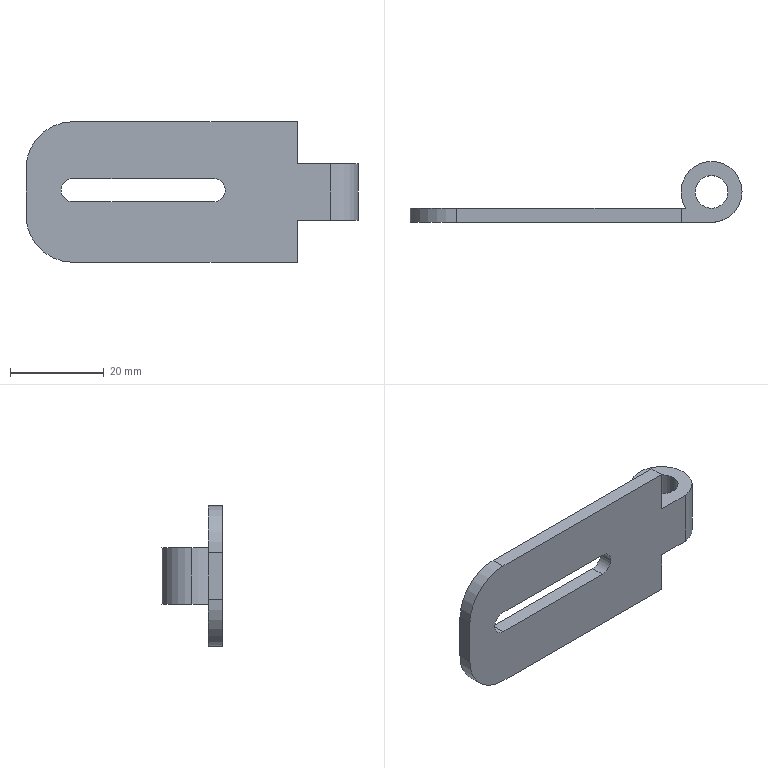Part | SolidWorks | features ICE 2, Extrusion 1, Fillet 1 | 1 solid | 20 faces | box 70.865 x 12.969 x 30 mm | volume 5794 mm3 | plane 11 | cylinder 9 | commonest cylinder face diameters 13 x3 5 x2 7 x2 20 x2
STEP:
#1=CARTESIAN_POINT('',(35.365,4.969,21.));
#2=VERTEX_POINT('',#1);
#3=CARTESIAN_POINT('',(28.365,4.969,21.));
#4=VERTEX_POINT('',#3);
#5=CARTESIAN_POINT('',(31.865,4.969,21.));
#6=DIRECTION('',(0.,0.,-1.));
#7=DIRECTION('',(-1.,0.,0.));
#8=AXIS2_PLACEMENT_3D('',#5,#6,#7);
#9=CIRCLE('',#8,3.5);
#10=EDGE_CURVE('',#2,#4,#9,.T.);
#11=ORIENTED_EDGE('',*,*,#10,.F.);
#12=CARTESIAN_POINT('',(35.365,4.969,9.));
#13=VERTEX_POINT('',#12);
#14=CARTESIAN_POINT('',(35.365,4.969,30.));
#15=DIRECTION('',(0.,0.,-1.));
#16=VECTOR('',#15,1000.);
#17=LINE('',#14,#16);
#18=EDGE_CURVE('',#2,#13,#17,.T.);
#19=ORIENTED_EDGE('',*,*,#18,.T.);
#20=CARTESIAN_POINT('',(28.365,4.969,9.));
#21=VERTEX_POINT('',#20);
#22=CARTESIAN_POINT('',(31.865,4.969,9.));
#23=DIRECTION('',(0.,0.,1.));
#24=DIRECTION('',(1.,0.,0.));
#25=AXIS2_PLACEMENT_3D('',#22,#23,#24);
#26=CIRCLE('',#25,3.5);
#27=EDGE_CURVE('',#21,#13,#26,.T.);
#28=ORIENTED_EDGE('',*,*,#27,.F.);
#29=CARTESIAN_POINT('',(28.365,4.969,30.));
#30=DIRECTION('',(0.,0.,-1.));
#31=VECTOR('',#30,1000.);
#32=LINE('',#29,#31);
#33=EDGE_CURVE('',#4,#21,#32,.T.);
#34=ORIENTED_EDGE('',*,*,#33,.F.);
#35=EDGE_LOOP('',(#11,#19,#28,#34));
#36=FACE_OUTER_BOUND('',#35,.T.);
#37=CARTESIAN_POINT('',(31.865,4.969,30.));
#38=DIRECTION('',(0.,0.,-1.));
#39=DIRECTION('',(-1.,0.,0.));
#40=AXIS2_PLACEMENT_3D('',#37,#38,#39);
#41=CYLINDRICAL_SURFACE('',#40,3.5);
#42=ADVANCED_FACE('',(#36),#41,.F.);
#43=CARTESIAN_POINT('',(25.365,4.969,21.));
#44=VERTEX_POINT('',#43);
#45=CARTESIAN_POINT('',(38.365,4.969,21.));
#46=VERTEX_POINT('',#45);
#47=CARTESIAN_POINT('',(31.865,4.969,21.));
#48=DIRECTION('',(0.,0.,-1.));
#49=DIRECTION('',(-1.,0.,0.));
#50=AXIS2_PLACEMENT_3D('',#47,#48,#49);
#51=CIRCLE('',#50,6.5);
#52=EDGE_CURVE('',#44,#46,#51,.T.);
#53=ORIENTED_EDGE('',*,*,#52,.T.);
#54=CARTESIAN_POINT('',(38.365,4.969,9.));
#55=VERTEX_POINT('',#54);
#56=CARTESIAN_POINT('',(38.365,4.969,30.));
#57=DIRECTION('',(0.,0.,-1.));
#58=VECTOR('',#57,1000.);
#59=LINE('',#56,#58);
#60=EDGE_CURVE('',#46,#55,#59,.T.);
#61=ORIENTED_EDGE('',*,*,#60,.T.);
#62=CARTESIAN_POINT('',(25.365,4.969,9.));
#63=VERTEX_POINT('',#62);
#64=CARTESIAN_POINT('',(31.865,4.969,9.));
#65=DIRECTION('',(0.,0.,1.));
#66=DIRECTION('',(1.,0.,0.));
#67=AXIS2_PLACEMENT_3D('',#64,#65,#66);
#68=CIRCLE('',#67,6.5);
#69=EDGE_CURVE('',#55,#63,#68,.T.);
#70=ORIENTED_EDGE('',*,*,#69,.T.);
#71=CARTESIAN_POINT('',(25.365,4.969,30.));
#72=DIRECTION('',(0.,0.,-1.));
#73=VECTOR('',#72,1000.);
#74=LINE('',#71,#73);
#75=EDGE_CURVE('',#44,#63,#74,.T.);
#76=ORIENTED_EDGE('',*,*,#75,.F.);
#77=EDGE_LOOP('',(#53,#61,#70,#76));
#78=FACE_OUTER_BOUND('',#77,.T.);
#79=CARTESIAN_POINT('',(31.865,4.969,30.));
#80=DIRECTION('',(0.,0.,-1.));
#81=DIRECTION('',(-1.,0.,0.));
#82=AXIS2_PLACEMENT_3D('',#79,#80,#81);
#83=CYLINDRICAL_SURFACE('',#82,6.5);
#84=ADVANCED_FACE('',(#78),#83,.T.);
#85=CARTESIAN_POINT('',(26.368,1.5,21.));
#86=VERTEX_POINT('',#85);
#87=CARTESIAN_POINT('',(31.865,4.969,21.));
#88=DIRECTION('',(0.,0.,-1.));
#89=DIRECTION('',(-1.,0.,0.));
#90=AXIS2_PLACEMENT_3D('',#87,#88,#89);
#91=CIRCLE('',#90,6.5);
#92=EDGE_CURVE('',#86,#44,#91,.T.);
#93=ORIENTED_EDGE('',*,*,#92,.T.);
#94=ORIENTED_EDGE('',*,*,#75,.T.);
#95=CARTESIAN_POINT('',(26.368,1.5,9.));
#96=VERTEX_POINT('',#95);
#97=CARTESIAN_POINT('',(31.865,4.969,9.));
#98=DIRECTION('',(0.,0.,1.));
#99=DIRECTION('',(1.,0.,0.));
#100=AXIS2_PLACEMENT_3D('',#97,#98,#99);
#101=CIRCLE('',#100,6.5);
#102=EDGE_CURVE('',#63,#96,#101,.T.);
#103=ORIENTED_EDGE('',*,*,#102,.T.);
#104=CARTESIAN_POINT('',(26.368,1.5,30.));
#105=DIRECTION('',(0.,0.,-1.));
#106=VECTOR('',#105,1000.);
#107=LINE('',#104,#106);
#108=EDGE_CURVE('',#86,#96,#107,.T.);
#109=ORIENTED_EDGE('',*,*,#108,.F.);
#110=EDGE_LOOP('',(#93,#94,#103,#109));
#111=FACE_OUTER_BOUND('',#110,.T.);
#112=CARTESIAN_POINT('',(31.865,4.969,30.));
#113=DIRECTION('',(0.,0.,-1.));
#114=DIRECTION('',(-1.,0.,0.));
#115=AXIS2_PLACEMENT_3D('',#112,#113,#114);
#116=CYLINDRICAL_SURFACE('',#115,6.5);
#117=ADVANCED_FACE('',(#111),#116,.T.);
#118=CARTESIAN_POINT('',(25.365,-1.5,30.));
#119=VERTEX_POINT('',#118);
#120=CARTESIAN_POINT('',(25.365,1.5,30.));
#121=VERTEX_POINT('',#120);
#122=CARTESIAN_POINT('',(25.365,-13.5,30.));
#123=DIRECTION('',(0.,1.,0.));
#124=VECTOR('',#123,1000.);
#125=LINE('',#122,#124);
#126=EDGE_CURVE('',#119,#121,#125,.T.);
#127=ORIENTED_EDGE('',*,*,#126,.T.);
#128=CARTESIAN_POINT('',(-22.5,1.5,30.));
#129=VERTEX_POINT('',#128);
#130=CARTESIAN_POINT('',(-32.5,1.5,30.));
#131=DIRECTION('',(-1.,0.,0.));
#132=VECTOR('',#131,1000.);
#133=LINE('',#130,#132);
#134=EDGE_CURVE('',#121,#129,#133,.T.);
#135=ORIENTED_EDGE('',*,*,#134,.T.);
#136=CARTESIAN_POINT('',(-22.5,-1.5,30.));
#137=VERTEX_POINT('',#136);
#138=CARTESIAN_POINT('',(-22.5,-1.5,30.));
#139=DIRECTION('',(0.,-1.,0.));
#140=VECTOR('',#139,1000.);
#141=LINE('',#138,#140);
#142=EDGE_CURVE('',#129,#137,#141,.T.);
#143=ORIENTED_EDGE('',*,*,#142,.T.);
#144=CARTESIAN_POINT('',(-32.5,-1.5,30.));
#145=DIRECTION('',(1.,0.,0.));
#146=VECTOR('',#145,1000.);
#147=LINE('',#144,#146);
#148=EDGE_CURVE('',#137,#119,#147,.T.);
#149=ORIENTED_EDGE('',*,*,#148,.T.);
#150=EDGE_LOOP('',(#127,#135,#143,#149));
#151=FACE_OUTER_BOUND('',#150,.T.);
#152=CARTESIAN_POINT('',(31.865,4.969,30.));
#153=DIRECTION('',(0.,0.,1.));
#154=DIRECTION('',(1.,0.,0.));
#155=AXIS2_PLACEMENT_3D('',#152,#153,#154);
#156=PLANE('',#155);
#157=ADVANCED_FACE('',(#151),#156,.T.);
#158=CARTESIAN_POINT('',(25.365,1.5,0.));
#159=VERTEX_POINT('',#158);
#160=CARTESIAN_POINT('',(-22.5,1.5,0.));
#161=VERTEX_POINT('',#160);
#162=CARTESIAN_POINT('',(-32.5,1.5,0.));
#163=DIRECTION('',(-1.,0.,0.));
#164=VECTOR('',#163,1000.);
#165=LINE('',#162,#164);
#166=EDGE_CURVE('',#159,#161,#165,.T.);
#167=ORIENTED_EDGE('',*,*,#166,.F.);
#168=CARTESIAN_POINT('',(25.365,-1.5,0.));
#169=VERTEX_POINT('',#168);
#170=CARTESIAN_POINT('',(25.365,-13.5,0.));
#171=DIRECTION('',(0.,1.,0.));
#172=VECTOR('',#171,1000.);
#173=LINE('',#170,#172);
#174=EDGE_CURVE('',#169,#159,#173,.T.);
#175=ORIENTED_EDGE('',*,*,#174,.F.);
#176=CARTESIAN_POINT('',(-22.5,-1.5,0.));
#177=VERTEX_POINT('',#176);
#178=CARTESIAN_POINT('',(-32.5,-1.5,0.));
#179=DIRECTION('',(1.,0.,0.));
#180=VECTOR('',#179,1000.);
#181=LINE('',#178,#180);
#182=EDGE_CURVE('',#177,#169,#181,.T.);
#183=ORIENTED_EDGE('',*,*,#182,.F.);
#184=CARTESIAN_POINT('',(-22.5,4.969,0.));
#185=DIRECTION('',(0.,1.,0.));
#186=VECTOR('',#185,1000.);
#187=LINE('',#184,#186);
#188=EDGE_CURVE('',#177,#161,#187,.T.);
#189=ORIENTED_EDGE('',*,*,#188,.T.);
#190=EDGE_LOOP('',(#167,#175,#183,#189));
#191=FACE_OUTER_BOUND('',#190,.T.);
#192=CARTESIAN_POINT('',(31.865,4.969,0.));
#193=DIRECTION('',(0.,0.,1.));
#194=DIRECTION('',(1.,0.,0.));
#195=AXIS2_PLACEMENT_3D('',#192,#193,#194);
#196=PLANE('',#195);
#197=ADVANCED_FACE('',(#191),#196,.F.);
#198=ORIENTED_EDGE('',*,*,#60,.F.);
#199=CARTESIAN_POINT('',(32.5,-1.5,21.));
#200=VERTEX_POINT('',#199);
#201=CARTESIAN_POINT('',(31.865,4.969,21.));
#202=DIRECTION('',(0.,0.,-1.));
#203=DIRECTION('',(-1.,0.,0.));
#204=AXIS2_PLACEMENT_3D('',#201,#202,#203);
#205=CIRCLE('',#204,6.5);
#206=EDGE_CURVE('',#46,#200,#205,.T.);
#207=ORIENTED_EDGE('',*,*,#206,.T.);
#208=CARTESIAN_POINT('',(32.5,-1.5,9.));
#209=VERTEX_POINT('',#208);
#210=CARTESIAN_POINT('',(32.5,-1.5,30.));
#211=DIRECTION('',(0.,0.,-1.));
#212=VECTOR('',#211,1000.);
#213=LINE('',#210,#212);
#214=EDGE_CURVE('',#200,#209,#213,.T.);
#215=ORIENTED_EDGE('',*,*,#214,.T.);
#216=CARTESIAN_POINT('',(31.865,4.969,9.));
#217=DIRECTION('',(0.,0.,1.));
#218=DIRECTION('',(1.,0.,0.));
#219=AXIS2_PLACEMENT_3D('',#216,#217,#218);
#220=CIRCLE('',#219,6.5);
#221=EDGE_CURVE('',#209,#55,#220,.T.);
#222=ORIENTED_EDGE('',*,*,#221,.T.);
#223=EDGE_LOOP('',(#198,#207,#215,#222));
#224=FACE_OUTER_BOUND('',#223,.T.);
#225=CARTESIAN_POINT('',(31.865,4.969,30.));
#226=DIRECTION('',(0.,0.,-1.));
#227=DIRECTION('',(-1.,0.,0.));
#228=AXIS2_PLACEMENT_3D('',#225,#226,#227);
#229=CYLINDRICAL_SURFACE('',#228,6.5);
#230=ADVANCED_FACE('',(#224),#229,.T.);
#231=CARTESIAN_POINT('',(7.5,1.5,12.878));
#232=VERTEX_POINT('',#231);
#233=CARTESIAN_POINT('',(-22.5,1.5,12.878));
#234=VERTEX_POINT('',#233);
#235=CARTESIAN_POINT('',(-22.5,1.5,12.878));
#236=DIRECTION('',(-1.,0.,0.));
#237=VECTOR('',#236,1000.);
#238=LINE('',#235,#237);
#239=EDGE_CURVE('',#232,#234,#238,.T.);
#240=ORIENTED_EDGE('',*,*,#239,.F.);
#241=CARTESIAN_POINT('',(7.5,1.5,17.878));
#242=VERTEX_POINT('',#241);
#243=CARTESIAN_POINT('',(7.5,1.5,15.378));
#244=DIRECTION('',(0.,1.,0.));
#245=DIRECTION('',(0.,0.,-1.));
#246=AXIS2_PLACEMENT_3D('',#243,#244,#245);
#247=CIRCLE('',#246,2.5);
#248=EDGE_CURVE('',#242,#232,#247,.T.);
#249=ORIENTED_EDGE('',*,*,#248,.F.);
#250=CARTESIAN_POINT('',(-22.5,1.5,17.878));
#251=VERTEX_POINT('',#250);
#252=CARTESIAN_POINT('',(-22.5,1.5,17.878));
#253=DIRECTION('',(1.,0.,0.));
#254=VECTOR('',#253,1000.);
#255=LINE('',#252,#254);
#256=EDGE_CURVE('',#251,#242,#255,.T.);
#257=ORIENTED_EDGE('',*,*,#256,.F.);
#258=CARTESIAN_POINT('',(-22.5,1.5,15.378));
#259=DIRECTION('',(0.,1.,0.));
#260=DIRECTION('',(0.,0.,-1.));
#261=AXIS2_PLACEMENT_3D('',#258,#259,#260);
#262=CIRCLE('',#261,2.5);
#263=EDGE_CURVE('',#234,#251,#262,.T.);
#264=ORIENTED_EDGE('',*,*,#263,.F.);
#265=EDGE_LOOP('',(#240,#249,#257,#264));
#266=FACE_BOUND('',#265,.T.);
#267=ORIENTED_EDGE('',*,*,#134,.F.);
#268=CARTESIAN_POINT('',(25.365,1.5,21.));
#269=VERTEX_POINT('',#268);
#270=CARTESIAN_POINT('',(25.365,1.5,30.));
#271=DIRECTION('',(0.,0.,-1.));
#272=VECTOR('',#271,1000.);
#273=LINE('',#270,#272);
#274=EDGE_CURVE('',#121,#269,#273,.T.);
#275=ORIENTED_EDGE('',*,*,#274,.T.);
#276=CARTESIAN_POINT('',(-32.5,1.5,21.));
#277=DIRECTION('',(1.,0.,0.));
#278=VECTOR('',#277,1000.);
#279=LINE('',#276,#278);
#280=EDGE_CURVE('',#269,#86,#279,.T.);
#281=ORIENTED_EDGE('',*,*,#280,.T.);
#282=ORIENTED_EDGE('',*,*,#108,.T.);
#283=CARTESIAN_POINT('',(25.365,1.5,9.));
#284=VERTEX_POINT('',#283);
#285=CARTESIAN_POINT('',(-32.5,1.5,9.));
#286=DIRECTION('',(-1.,0.,0.));
#287=VECTOR('',#286,1000.);
#288=LINE('',#285,#287);
#289=EDGE_CURVE('',#96,#284,#288,.T.);
#290=ORIENTED_EDGE('',*,*,#289,.T.);
#291=CARTESIAN_POINT('',(25.365,1.5,30.));
#292=DIRECTION('',(0.,0.,-1.));
#293=VECTOR('',#292,1000.);
#294=LINE('',#291,#293);
#295=EDGE_CURVE('',#284,#159,#294,.T.);
#296=ORIENTED_EDGE('',*,*,#295,.T.);
#297=ORIENTED_EDGE('',*,*,#166,.T.);
#298=CARTESIAN_POINT('',(-32.5,1.5,10.));
#299=VERTEX_POINT('',#298);
#300=CARTESIAN_POINT('',(-22.5,1.5,10.));
#301=DIRECTION('',(0.,1.,0.));
#302=DIRECTION('',(0.,0.,-1.));
#303=AXIS2_PLACEMENT_3D('',#300,#301,#302);
#304=CIRCLE('',#303,10.);
#305=EDGE_CURVE('',#161,#299,#304,.T.);
#306=ORIENTED_EDGE('',*,*,#305,.T.);
#307=CARTESIAN_POINT('',(-32.5,1.5,20.));
#308=VERTEX_POINT('',#307);
#309=CARTESIAN_POINT('',(-32.5,1.5,30.));
#310=DIRECTION('',(0.,0.,-1.));
#311=VECTOR('',#310,1000.);
#312=LINE('',#309,#311);
#313=EDGE_CURVE('',#308,#299,#312,.T.);
#314=ORIENTED_EDGE('',*,*,#313,.F.);
#315=CARTESIAN_POINT('',(-22.5,1.5,20.));
#316=DIRECTION('',(0.,1.,0.));
#317=DIRECTION('',(0.,0.,-1.));
#318=AXIS2_PLACEMENT_3D('',#315,#316,#317);
#319=CIRCLE('',#318,10.);
#320=EDGE_CURVE('',#308,#129,#319,.T.);
#321=ORIENTED_EDGE('',*,*,#320,.T.);
#322=EDGE_LOOP('',(#267,#275,#281,#282,#290,#296,#297,#306,#314,#321));
#323=FACE_OUTER_BOUND('',#322,.T.);
#324=CARTESIAN_POINT('',(-32.5,1.5,30.));
#325=DIRECTION('',(0.,-1.,0.));
#326=DIRECTION('',(0.,0.,-1.));
#327=AXIS2_PLACEMENT_3D('',#324,#325,#326);
#328=PLANE('',#327);
#329=ADVANCED_FACE('',(#266,#323),#328,.F.);
#330=ORIENTED_EDGE('',*,*,#313,.T.);
#331=CARTESIAN_POINT('',(-32.5,-1.5,10.));
#332=VERTEX_POINT('',#331);
#333=CARTESIAN_POINT('',(-32.5,1.5,10.));
#334=DIRECTION('',(0.,-1.,0.));
#335=VECTOR('',#334,1000.);
#336=LINE('',#333,#335);
#337=EDGE_CURVE('',#299,#332,#336,.T.);
#338=ORIENTED_EDGE('',*,*,#337,.T.);
#339=CARTESIAN_POINT('',(-32.5,-1.5,20.));
#340=VERTEX_POINT('',#339);
#341=CARTESIAN_POINT('',(-32.5,-1.5,30.));
#342=DIRECTION('',(0.,0.,-1.));
#343=VECTOR('',#342,1000.);
#344=LINE('',#341,#343);
#345=EDGE_CURVE('',#340,#332,#344,.T.);
#346=ORIENTED_EDGE('',*,*,#345,.F.);
#347=CARTESIAN_POINT('',(-32.5,1.5,20.));
#348=DIRECTION('',(0.,1.,0.));
#349=VECTOR('',#348,1000.);
#350=LINE('',#347,#349);
#351=EDGE_CURVE('',#340,#308,#350,.T.);
#352=ORIENTED_EDGE('',*,*,#351,.T.);
#353=EDGE_LOOP('',(#330,#338,#346,#352));
#354=FACE_OUTER_BOUND('',#353,.T.);
#355=CARTESIAN_POINT('',(-32.5,1.5,30.));
#356=DIRECTION('',(1.,0.,0.));
#357=DIRECTION('',(0.,0.,-1.));
#358=AXIS2_PLACEMENT_3D('',#355,#356,#357);
#359=PLANE('',#358);
#360=ADVANCED_FACE('',(#354),#359,.F.);
#361=CARTESIAN_POINT('',(-22.5,-1.5,17.878));
#362=VERTEX_POINT('',#361);
#363=CARTESIAN_POINT('',(7.5,-1.5,17.878));
#364=VERTEX_POINT('',#363);
#365=CARTESIAN_POINT('',(-32.5,-1.5,17.878));
#366=DIRECTION('',(1.,0.,0.));
#367=VECTOR('',#366,1000.);
#368=LINE('',#365,#367);
#369=EDGE_CURVE('',#362,#364,#368,.T.);
#370=ORIENTED_EDGE('',*,*,#369,.T.);
#371=CARTESIAN_POINT('',(7.5,-1.5,12.878));
#372=VERTEX_POINT('',#371);
#373=CARTESIAN_POINT('',(7.5,-1.5,15.378));
#374=DIRECTION('',(0.,1.,0.));
#375=DIRECTION('',(0.,0.,1.));
#376=AXIS2_PLACEMENT_3D('',#373,#374,#375);
#377=CIRCLE('',#376,2.5);
#378=EDGE_CURVE('',#364,#372,#377,.T.);
#379=ORIENTED_EDGE('',*,*,#378,.T.);
#380=CARTESIAN_POINT('',(-22.5,-1.5,12.878));
#381=VERTEX_POINT('',#380);
#382=CARTESIAN_POINT('',(-32.5,-1.5,12.878));
#383=DIRECTION('',(-1.,0.,0.));
#384=VECTOR('',#383,1000.);
#385=LINE('',#382,#384);
#386=EDGE_CURVE('',#372,#381,#385,.T.);
#387=ORIENTED_EDGE('',*,*,#386,.T.);
#388=CARTESIAN_POINT('',(-22.5,-1.5,15.378));
#389=DIRECTION('',(0.,1.,0.));
#390=DIRECTION('',(0.,0.,1.));
#391=AXIS2_PLACEMENT_3D('',#388,#389,#390);
#392=CIRCLE('',#391,2.5);
#393=EDGE_CURVE('',#381,#362,#392,.T.);
#394=ORIENTED_EDGE('',*,*,#393,.T.);
#395=EDGE_LOOP('',(#370,#379,#387,#394));
#396=FACE_BOUND('',#395,.T.);
#397=CARTESIAN_POINT('',(25.365,-1.5,21.));
#398=VERTEX_POINT('',#397);
#399=CARTESIAN_POINT('',(-32.5,-1.5,21.));
#400=DIRECTION('',(-1.,0.,0.));
#401=VECTOR('',#400,1000.);
#402=LINE('',#399,#401);
#403=EDGE_CURVE('',#200,#398,#402,.T.);
#404=ORIENTED_EDGE('',*,*,#403,.T.);
#405=CARTESIAN_POINT('',(25.365,-1.5,30.));
#406=DIRECTION('',(0.,0.,1.));
#407=VECTOR('',#406,1000.);
#408=LINE('',#405,#407);
#409=EDGE_CURVE('',#398,#119,#408,.T.);
#410=ORIENTED_EDGE('',*,*,#409,.T.);
#411=ORIENTED_EDGE('',*,*,#148,.F.);
#412=CARTESIAN_POINT('',(-22.5,-1.5,20.));
#413=DIRECTION('',(0.,-1.,0.));
#414=DIRECTION('',(0.,0.,1.));
#415=AXIS2_PLACEMENT_3D('',#412,#413,#414);
#416=CIRCLE('',#415,10.);
#417=EDGE_CURVE('',#137,#340,#416,.T.);
#418=ORIENTED_EDGE('',*,*,#417,.T.);
#419=ORIENTED_EDGE('',*,*,#345,.T.);
#420=CARTESIAN_POINT('',(-22.5,-1.5,10.));
#421=DIRECTION('',(0.,-1.,0.));
#422=DIRECTION('',(0.,0.,1.));
#423=AXIS2_PLACEMENT_3D('',#420,#421,#422);
#424=CIRCLE('',#423,10.);
#425=EDGE_CURVE('',#332,#177,#424,.T.);
#426=ORIENTED_EDGE('',*,*,#425,.T.);
#427=ORIENTED_EDGE('',*,*,#182,.T.);
#428=CARTESIAN_POINT('',(25.365,-1.5,9.));
#429=VERTEX_POINT('',#428);
#430=CARTESIAN_POINT('',(25.365,-1.5,30.));
#431=DIRECTION('',(0.,0.,1.));
#432=VECTOR('',#431,1000.);
#433=LINE('',#430,#432);
#434=EDGE_CURVE('',#169,#429,#433,.T.);
#435=ORIENTED_EDGE('',*,*,#434,.T.);
#436=CARTESIAN_POINT('',(-32.5,-1.5,9.));
#437=DIRECTION('',(1.,0.,0.));
#438=VECTOR('',#437,1000.);
#439=LINE('',#436,#438);
#440=EDGE_CURVE('',#429,#209,#439,.T.);
#441=ORIENTED_EDGE('',*,*,#440,.T.);
#442=ORIENTED_EDGE('',*,*,#214,.F.);
#443=EDGE_LOOP('',(#404,#410,#411,#418,#419,#426,#427,#435,#441,#442));
#444=FACE_OUTER_BOUND('',#443,.T.);
#445=CARTESIAN_POINT('',(-32.5,-1.5,30.));
#446=DIRECTION('',(0.,1.,0.));
#447=DIRECTION('',(0.,0.,1.));
#448=AXIS2_PLACEMENT_3D('',#445,#446,#447);
#449=PLANE('',#448);
#450=ADVANCED_FACE('',(#396,#444),#449,.F.);
#451=ORIENTED_EDGE('',*,*,#305,.F.);
#452=ORIENTED_EDGE('',*,*,#188,.F.);
#453=ORIENTED_EDGE('',*,*,#425,.F.);
#454=ORIENTED_EDGE('',*,*,#337,.F.);
#455=EDGE_LOOP('',(#451,#452,#453,#454));
#456=FACE_OUTER_BOUND('',#455,.T.);
#457=CARTESIAN_POINT('',(-22.5,1.5,10.));
#458=DIRECTION('',(0.,-1.,0.));
#459=DIRECTION('',(0.,0.,-1.));
#460=AXIS2_PLACEMENT_3D('',#457,#458,#459);
#461=CYLINDRICAL_SURFACE('',#460,10.);
#462=ADVANCED_FACE('',(#456),#461,.T.);
#463=ORIENTED_EDGE('',*,*,#320,.F.);
#464=ORIENTED_EDGE('',*,*,#351,.F.);
#465=ORIENTED_EDGE('',*,*,#417,.F.);
#466=ORIENTED_EDGE('',*,*,#142,.F.);
#467=EDGE_LOOP('',(#463,#464,#465,#466));
#468=FACE_OUTER_BOUND('',#467,.T.);
#469=CARTESIAN_POINT('',(-22.5,4.969,20.));
#470=DIRECTION('',(0.,1.,0.));
#471=DIRECTION('',(0.,0.,1.));
#472=AXIS2_PLACEMENT_3D('',#469,#470,#471);
#473=CYLINDRICAL_SURFACE('',#472,10.);
#474=ADVANCED_FACE('',(#468),#473,.T.);
#475=CARTESIAN_POINT('',(7.5,-28.5,17.878));
#476=DIRECTION('',(0.,1.,0.));
#477=VECTOR('',#476,1000.);
#478=LINE('',#475,#477);
#479=EDGE_CURVE('',#364,#242,#478,.T.);
#480=ORIENTED_EDGE('',*,*,#479,.T.);
#481=ORIENTED_EDGE('',*,*,#248,.T.);
#482=CARTESIAN_POINT('',(7.5,-28.5,12.878));
#483=DIRECTION('',(0.,1.,0.));
#484=VECTOR('',#483,1000.);
#485=LINE('',#482,#484);
#486=EDGE_CURVE('',#372,#232,#485,.T.);
#487=ORIENTED_EDGE('',*,*,#486,.F.);
#488=ORIENTED_EDGE('',*,*,#378,.F.);
#489=EDGE_LOOP('',(#480,#481,#487,#488));
#490=FACE_OUTER_BOUND('',#489,.T.);
#491=CARTESIAN_POINT('',(7.5,-28.5,15.378));
#492=DIRECTION('',(0.,1.,0.));
#493=DIRECTION('',(0.,0.,1.));
#494=AXIS2_PLACEMENT_3D('',#491,#492,#493);
#495=CYLINDRICAL_SURFACE('',#494,2.5);
#496=ADVANCED_FACE('',(#490),#495,.F.);
#497=CARTESIAN_POINT('',(-22.5,-28.5,17.878));
#498=DIRECTION('',(0.,1.,0.));
#499=VECTOR('',#498,1000.);
#500=LINE('',#497,#499);
#501=EDGE_CURVE('',#362,#251,#500,.T.);
#502=ORIENTED_EDGE('',*,*,#501,.T.);
#503=ORIENTED_EDGE('',*,*,#256,.T.);
#504=ORIENTED_EDGE('',*,*,#479,.F.);
#505=ORIENTED_EDGE('',*,*,#369,.F.);
#506=EDGE_LOOP('',(#502,#503,#504,#505));
#507=FACE_OUTER_BOUND('',#506,.T.);
#508=CARTESIAN_POINT('',(-22.5,-28.5,17.878));
#509=DIRECTION('',(0.,0.,1.));
#510=DIRECTION('',(1.,0.,0.));
#511=AXIS2_PLACEMENT_3D('',#508,#509,#510);
#512=PLANE('',#511);
#513=ADVANCED_FACE('',(#507),#512,.F.);
#514=CARTESIAN_POINT('',(-22.5,-28.5,12.878));
#515=DIRECTION('',(0.,1.,0.));
#516=VECTOR('',#515,1000.);
#517=LINE('',#514,#516);
#518=EDGE_CURVE('',#381,#234,#517,.T.);
#519=ORIENTED_EDGE('',*,*,#518,.T.);
#520=ORIENTED_EDGE('',*,*,#263,.T.);
#521=ORIENTED_EDGE('',*,*,#501,.F.);
#522=ORIENTED_EDGE('',*,*,#393,.F.);
#523=EDGE_LOOP('',(#519,#520,#521,#522));
#524=FACE_OUTER_BOUND('',#523,.T.);
#525=CARTESIAN_POINT('',(-22.5,-28.5,15.378));
#526=DIRECTION('',(0.,1.,0.));
#527=DIRECTION('',(0.,0.,1.));
#528=AXIS2_PLACEMENT_3D('',#525,#526,#527);
#529=CYLINDRICAL_SURFACE('',#528,2.5);
#530=ADVANCED_FACE('',(#524),#529,.F.);
#531=ORIENTED_EDGE('',*,*,#486,.T.);
#532=ORIENTED_EDGE('',*,*,#239,.T.);
#533=ORIENTED_EDGE('',*,*,#518,.F.);
#534=ORIENTED_EDGE('',*,*,#386,.F.);
#535=EDGE_LOOP('',(#531,#532,#533,#534));
#536=FACE_OUTER_BOUND('',#535,.T.);
#537=CARTESIAN_POINT('',(-22.5,-28.5,12.878));
#538=DIRECTION('',(0.,0.,-1.));
#539=DIRECTION('',(-1.,0.,0.));
#540=AXIS2_PLACEMENT_3D('',#537,#538,#539);
#541=PLANE('',#540);
#542=ADVANCED_FACE('',(#536),#541,.F.);
#543=CARTESIAN_POINT('',(25.365,-13.5,9.));
#544=DIRECTION('',(0.,1.,0.));
#545=VECTOR('',#544,1000.);
#546=LINE('',#543,#545);
#547=EDGE_CURVE('',#429,#284,#546,.T.);
#548=ORIENTED_EDGE('',*,*,#547,.F.);
#549=ORIENTED_EDGE('',*,*,#434,.F.);
#550=ORIENTED_EDGE('',*,*,#174,.T.);
#551=ORIENTED_EDGE('',*,*,#295,.F.);
#552=EDGE_LOOP('',(#548,#549,#550,#551));
#553=FACE_OUTER_BOUND('',#552,.T.);
#554=CARTESIAN_POINT('',(25.365,-13.5,0.));
#555=DIRECTION('',(-1.,0.,0.));
#556=DIRECTION('',(0.,0.,1.));
#557=AXIS2_PLACEMENT_3D('',#554,#555,#556);
#558=PLANE('',#557);
#559=ADVANCED_FACE('',(#553),#558,.F.);
#560=ORIENTED_EDGE('',*,*,#27,.T.);
#561=CARTESIAN_POINT('',(31.865,4.969,9.));
#562=DIRECTION('',(0.,0.,1.));
#563=DIRECTION('',(1.,0.,0.));
#564=AXIS2_PLACEMENT_3D('',#561,#562,#563);
#565=CIRCLE('',#564,3.5);
#566=EDGE_CURVE('',#13,#21,#565,.T.);
#567=ORIENTED_EDGE('',*,*,#566,.T.);
#568=EDGE_LOOP('',(#560,#567));
#569=FACE_BOUND('',#568,.T.);
#570=ORIENTED_EDGE('',*,*,#221,.F.);
#571=ORIENTED_EDGE('',*,*,#440,.F.);
#572=ORIENTED_EDGE('',*,*,#547,.T.);
#573=ORIENTED_EDGE('',*,*,#289,.F.);
#574=ORIENTED_EDGE('',*,*,#102,.F.);
#575=ORIENTED_EDGE('',*,*,#69,.F.);
#576=EDGE_LOOP('',(#570,#571,#572,#573,#574,#575));
#577=FACE_OUTER_BOUND('',#576,.T.);
#578=CARTESIAN_POINT('',(25.365,-13.5,9.));
#579=DIRECTION('',(0.,0.,1.));
#580=DIRECTION('',(1.,0.,0.));
#581=AXIS2_PLACEMENT_3D('',#578,#579,#580);
#582=PLANE('',#581);
#583=ADVANCED_FACE('',(#569,#577),#582,.F.);
#584=ORIENTED_EDGE('',*,*,#126,.F.);
#585=ORIENTED_EDGE('',*,*,#409,.F.);
#586=CARTESIAN_POINT('',(25.365,-13.5,21.));
#587=DIRECTION('',(0.,1.,0.));
#588=VECTOR('',#587,1000.);
#589=LINE('',#586,#588);
#590=EDGE_CURVE('',#398,#269,#589,.T.);
#591=ORIENTED_EDGE('',*,*,#590,.T.);
#592=ORIENTED_EDGE('',*,*,#274,.F.);
#593=EDGE_LOOP('',(#584,#585,#591,#592));
#594=FACE_OUTER_BOUND('',#593,.T.);
#595=CARTESIAN_POINT('',(25.365,-13.5,21.));
#596=DIRECTION('',(-1.,0.,0.));
#597=DIRECTION('',(0.,0.,1.));
#598=AXIS2_PLACEMENT_3D('',#595,#596,#597);
#599=PLANE('',#598);
#600=ADVANCED_FACE('',(#594),#599,.F.);
#601=CARTESIAN_POINT('',(31.865,4.969,21.));
#602=DIRECTION('',(0.,0.,-1.));
#603=DIRECTION('',(-1.,0.,0.));
#604=AXIS2_PLACEMENT_3D('',#601,#602,#603);
#605=CIRCLE('',#604,3.5);
#606=EDGE_CURVE('',#4,#2,#605,.T.);
#607=ORIENTED_EDGE('',*,*,#606,.T.);
#608=ORIENTED_EDGE('',*,*,#10,.T.);
#609=EDGE_LOOP('',(#607,#608));
#610=FACE_BOUND('',#609,.T.);
#611=ORIENTED_EDGE('',*,*,#590,.F.);
#612=ORIENTED_EDGE('',*,*,#403,.F.);
#613=ORIENTED_EDGE('',*,*,#206,.F.);
#614=ORIENTED_EDGE('',*,*,#52,.F.);
#615=ORIENTED_EDGE('',*,*,#92,.F.);
#616=ORIENTED_EDGE('',*,*,#280,.F.);
#617=EDGE_LOOP('',(#611,#612,#613,#614,#615,#616));
#618=FACE_OUTER_BOUND('',#617,.T.);
#619=CARTESIAN_POINT('',(25.365,-13.5,21.));
#620=DIRECTION('',(0.,0.,-1.));
#621=DIRECTION('',(-1.,0.,0.));
#622=AXIS2_PLACEMENT_3D('',#619,#620,#621);
#623=PLANE('',#622);
#624=ADVANCED_FACE('',(#610,#618),#623,.F.);
#625=ORIENTED_EDGE('',*,*,#18,.F.);
#626=ORIENTED_EDGE('',*,*,#606,.F.);
#627=ORIENTED_EDGE('',*,*,#33,.T.);
#628=ORIENTED_EDGE('',*,*,#566,.F.);
#629=EDGE_LOOP('',(#625,#626,#627,#628));
#630=FACE_OUTER_BOUND('',#629,.T.);
#631=CARTESIAN_POINT('',(31.865,4.969,30.));
#632=DIRECTION('',(0.,0.,-1.));
#633=DIRECTION('',(-1.,0.,0.));
#634=AXIS2_PLACEMENT_3D('',#631,#632,#633);
#635=CYLINDRICAL_SURFACE('',#634,3.5);
#636=ADVANCED_FACE('',(#630),#635,.F.);
#637=CLOSED_SHELL('',(#42,#84,#117,#157,#197,#230,#329,#360,#450,#462,#474,#496,#513,#530,#542,#559,#583,#600,#624,#636));
#638=MANIFOLD_SOLID_BREP('',#637);
#639=CARTESIAN_POINT('',(0.,0.,0.));
#640=DIRECTION('',(0.,0.,1.));
#641=DIRECTION('',(1.,0.,0.));
#642=AXIS2_PLACEMENT_3D('',#639,#640,#641);
#643=(LENGTH_UNIT()NAMED_UNIT(*)SI_UNIT(.MILLI.,.METRE.));
#644=UNCERTAINTY_MEASURE_WITH_UNIT(LENGTH_MEASURE(0.00001),#643,'','');
#645=(NAMED_UNIT(*)PLANE_ANGLE_UNIT()SI_UNIT($,.RADIAN.));
#646=(NAMED_UNIT(*)SI_UNIT($,.STERADIAN.)SOLID_ANGLE_UNIT());
#647=(GEOMETRIC_REPRESENTATION_CONTEXT(3)GLOBAL_UNCERTAINTY_ASSIGNED_CONTEXT((#644))GLOBAL_UNIT_ASSIGNED_CONTEXT((#643,#645,#646))REPRESENTATION_CONTEXT('',''));
#648=ADVANCED_BREP_SHAPE_REPRESENTATION('',(#638,#642),#647);